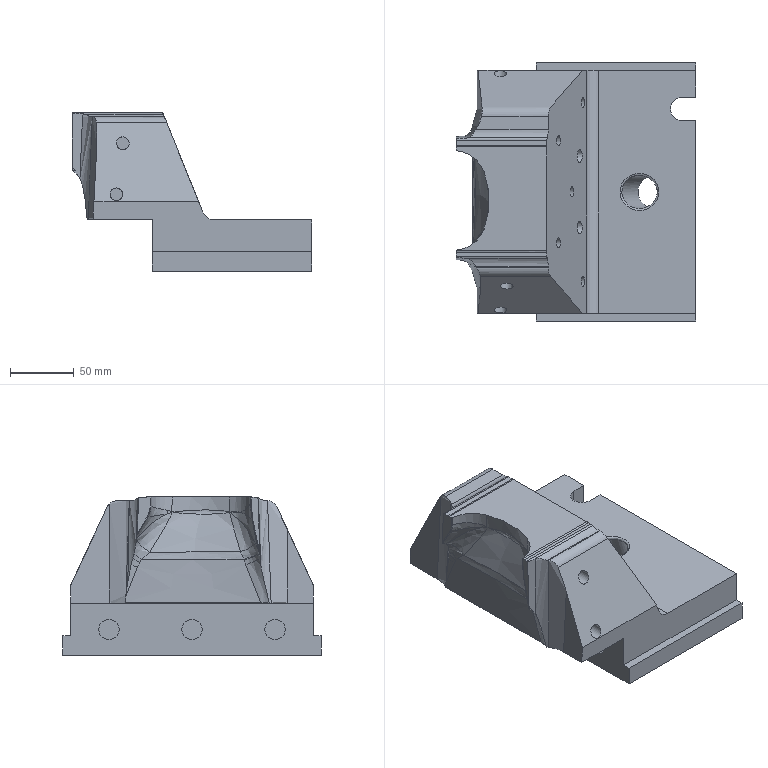Part | STEP file | solid 158 | 1 solid | 198 faces | box 187.742 x 202 x 123.694 mm | volume 1808093 mm3 | plane 92 | spline 41 | cylinder 40 | other 13 | cone 12 | commonest cylinder face diameters 10 x16 6.7 x5 8 x5 16 x5 20 x3 5.527 x2